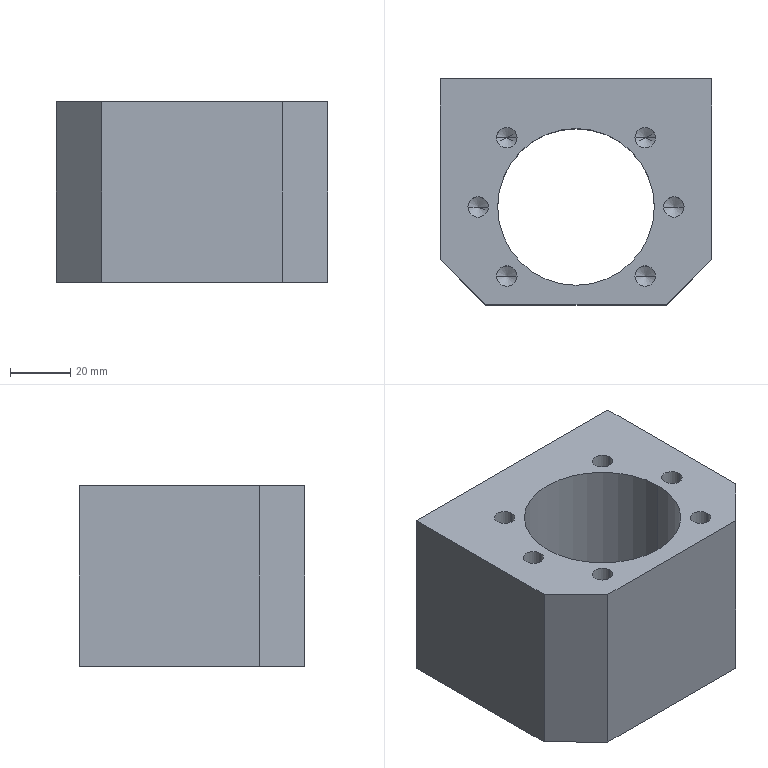Part | SolidWorks | features 3DProfileFeature 2, HoleWzd 2, Chamfer 1, Extrusion 1 | 1 solid | 50 faces | box 90 x 75 x 60 mm | volume 256657 mm3 | cylinder 22 | cone 20 | plane 8 | commonest cylinder face diameters 6.8 x20 52 x2
STEP:
#1=CARTESIAN_POINT('',(32.5,22.75,-23.4));
#2=VERTEX_POINT('',#1);
#3=CARTESIAN_POINT('',(32.5,22.75,-16.6));
#4=VERTEX_POINT('',#3);
#5=CARTESIAN_POINT('',(32.5,22.75,-20.));
#6=DIRECTION('',(0.,1.,0.));
#7=DIRECTION('',(0.,0.,1.));
#8=AXIS2_PLACEMENT_3D('',#5,#6,#7);
#9=CIRCLE('',#8,3.4);
#10=EDGE_CURVE('',#2,#4,#9,.T.);
#11=ORIENTED_EDGE('',*,*,#10,.F.);
#12=CARTESIAN_POINT('',(32.5,42.5,-23.4));
#13=VERTEX_POINT('',#12);
#14=CARTESIAN_POINT('',(32.5,42.5,-23.4));
#15=DIRECTION('',(0.,1.,0.));
#16=VECTOR('',#15,1000.);
#17=LINE('',#14,#16);
#18=EDGE_CURVE('',#2,#13,#17,.T.);
#19=ORIENTED_EDGE('',*,*,#18,.T.);
#20=CARTESIAN_POINT('',(32.5,42.5,-16.6));
#21=VERTEX_POINT('',#20);
#22=CARTESIAN_POINT('',(32.5,42.5,-20.));
#23=DIRECTION('',(0.,1.,0.));
#24=DIRECTION('',(0.,0.,1.));
#25=AXIS2_PLACEMENT_3D('',#22,#23,#24);
#26=CIRCLE('',#25,3.4);
#27=EDGE_CURVE('',#13,#21,#26,.T.);
#28=ORIENTED_EDGE('',*,*,#27,.T.);
#29=CARTESIAN_POINT('',(32.5,42.5,-16.6));
#30=DIRECTION('',(0.,1.,0.));
#31=VECTOR('',#30,1000.);
#32=LINE('',#29,#31);
#33=EDGE_CURVE('',#4,#21,#32,.T.);
#34=ORIENTED_EDGE('',*,*,#33,.F.);
#35=EDGE_LOOP('',(#11,#19,#28,#34));
#36=FACE_OUTER_BOUND('',#35,.T.);
#37=CARTESIAN_POINT('',(32.5,42.5,-20.));
#38=DIRECTION('',(0.,1.,0.));
#39=DIRECTION('',(0.,0.,1.));
#40=AXIS2_PLACEMENT_3D('',#37,#38,#39);
#41=CYLINDRICAL_SURFACE('',#40,3.4);
#42=ADVANCED_FACE('',(#36),#41,.F.);
#43=CARTESIAN_POINT('',(32.5,20.707,-20.));
#44=VERTEX_POINT('',#43);
#45=CARTESIAN_POINT('',(32.5,22.75,-16.6));
#46=DIRECTION('',(0.,0.515,0.8572));
#47=VECTOR('',#46,1000.);
#48=LINE('',#45,#47);
#49=EDGE_CURVE('',#44,#4,#48,.T.);
#50=ORIENTED_EDGE('',*,*,#49,.F.);
#51=CARTESIAN_POINT('',(32.5,22.75,-23.4));
#52=DIRECTION('',(0.,0.515,-0.8572));
#53=VECTOR('',#52,1000.);
#54=LINE('',#51,#53);
#55=EDGE_CURVE('',#44,#2,#54,.T.);
#56=ORIENTED_EDGE('',*,*,#55,.T.);
#57=ORIENTED_EDGE('',*,*,#10,.T.);
#58=EDGE_LOOP('',(#50,#56,#57));
#59=FACE_OUTER_BOUND('',#58,.T.);
#60=CARTESIAN_POINT('',(32.5,22.75,-20.));
#61=DIRECTION('',(0.,1.,0.));
#62=DIRECTION('',(0.,0.,1.));
#63=AXIS2_PLACEMENT_3D('',#60,#61,#62);
#64=CONICAL_SURFACE('',#63,3.4,1.03);
#65=ADVANCED_FACE('',(#59),#64,.F.);
#66=CARTESIAN_POINT('',(32.5,22.75,16.6));
#67=VERTEX_POINT('',#66);
#68=CARTESIAN_POINT('',(32.5,22.75,23.4));
#69=VERTEX_POINT('',#68);
#70=CARTESIAN_POINT('',(32.5,22.75,20.));
#71=DIRECTION('',(0.,1.,0.));
#72=DIRECTION('',(0.,0.,1.));
#73=AXIS2_PLACEMENT_3D('',#70,#71,#72);
#74=CIRCLE('',#73,3.4);
#75=EDGE_CURVE('',#67,#69,#74,.T.);
#76=ORIENTED_EDGE('',*,*,#75,.F.);
#77=CARTESIAN_POINT('',(32.5,42.5,16.6));
#78=VERTEX_POINT('',#77);
#79=CARTESIAN_POINT('',(32.5,42.5,16.6));
#80=DIRECTION('',(0.,1.,0.));
#81=VECTOR('',#80,1000.);
#82=LINE('',#79,#81);
#83=EDGE_CURVE('',#67,#78,#82,.T.);
#84=ORIENTED_EDGE('',*,*,#83,.T.);
#85=CARTESIAN_POINT('',(32.5,42.5,23.4));
#86=VERTEX_POINT('',#85);
#87=CARTESIAN_POINT('',(32.5,42.5,20.));
#88=DIRECTION('',(0.,1.,0.));
#89=DIRECTION('',(0.,0.,1.));
#90=AXIS2_PLACEMENT_3D('',#87,#88,#89);
#91=CIRCLE('',#90,3.4);
#92=EDGE_CURVE('',#78,#86,#91,.T.);
#93=ORIENTED_EDGE('',*,*,#92,.T.);
#94=CARTESIAN_POINT('',(32.5,42.5,23.4));
#95=DIRECTION('',(0.,1.,0.));
#96=VECTOR('',#95,1000.);
#97=LINE('',#94,#96);
#98=EDGE_CURVE('',#69,#86,#97,.T.);
#99=ORIENTED_EDGE('',*,*,#98,.F.);
#100=EDGE_LOOP('',(#76,#84,#93,#99));
#101=FACE_OUTER_BOUND('',#100,.T.);
#102=CARTESIAN_POINT('',(32.5,42.5,20.));
#103=DIRECTION('',(0.,1.,0.));
#104=DIRECTION('',(0.,0.,1.));
#105=AXIS2_PLACEMENT_3D('',#102,#103,#104);
#106=CYLINDRICAL_SURFACE('',#105,3.4);
#107=ADVANCED_FACE('',(#101),#106,.F.);
#108=CARTESIAN_POINT('',(32.5,20.707,20.));
#109=VERTEX_POINT('',#108);
#110=CARTESIAN_POINT('',(32.5,22.75,23.4));
#111=DIRECTION('',(0.,0.515,0.8572));
#112=VECTOR('',#111,1000.);
#113=LINE('',#110,#112);
#114=EDGE_CURVE('',#109,#69,#113,.T.);
#115=ORIENTED_EDGE('',*,*,#114,.F.);
#116=CARTESIAN_POINT('',(32.5,22.75,16.6));
#117=DIRECTION('',(0.,0.515,-0.8572));
#118=VECTOR('',#117,1000.);
#119=LINE('',#116,#118);
#120=EDGE_CURVE('',#109,#67,#119,.T.);
#121=ORIENTED_EDGE('',*,*,#120,.T.);
#122=ORIENTED_EDGE('',*,*,#75,.T.);
#123=EDGE_LOOP('',(#115,#121,#122));
#124=FACE_OUTER_BOUND('',#123,.T.);
#125=CARTESIAN_POINT('',(32.5,22.75,20.));
#126=DIRECTION('',(0.,1.,0.));
#127=DIRECTION('',(0.,0.,1.));
#128=AXIS2_PLACEMENT_3D('',#125,#126,#127);
#129=CONICAL_SURFACE('',#128,3.4,1.03);
#130=ADVANCED_FACE('',(#124),#129,.F.);
#131=CARTESIAN_POINT('',(-32.5,22.75,16.6));
#132=VERTEX_POINT('',#131);
#133=CARTESIAN_POINT('',(-32.5,22.75,23.4));
#134=VERTEX_POINT('',#133);
#135=CARTESIAN_POINT('',(-32.5,22.75,20.));
#136=DIRECTION('',(0.,1.,0.));
#137=DIRECTION('',(0.,0.,1.));
#138=AXIS2_PLACEMENT_3D('',#135,#136,#137);
#139=CIRCLE('',#138,3.4);
#140=EDGE_CURVE('',#132,#134,#139,.T.);
#141=ORIENTED_EDGE('',*,*,#140,.F.);
#142=CARTESIAN_POINT('',(-32.5,42.5,16.6));
#143=VERTEX_POINT('',#142);
#144=CARTESIAN_POINT('',(-32.5,42.5,16.6));
#145=DIRECTION('',(0.,1.,0.));
#146=VECTOR('',#145,1000.);
#147=LINE('',#144,#146);
#148=EDGE_CURVE('',#132,#143,#147,.T.);
#149=ORIENTED_EDGE('',*,*,#148,.T.);
#150=CARTESIAN_POINT('',(-32.5,42.5,23.4));
#151=VERTEX_POINT('',#150);
#152=CARTESIAN_POINT('',(-32.5,42.5,20.));
#153=DIRECTION('',(0.,1.,0.));
#154=DIRECTION('',(0.,0.,1.));
#155=AXIS2_PLACEMENT_3D('',#152,#153,#154);
#156=CIRCLE('',#155,3.4);
#157=EDGE_CURVE('',#143,#151,#156,.T.);
#158=ORIENTED_EDGE('',*,*,#157,.T.);
#159=CARTESIAN_POINT('',(-32.5,42.5,23.4));
#160=DIRECTION('',(0.,1.,0.));
#161=VECTOR('',#160,1000.);
#162=LINE('',#159,#161);
#163=EDGE_CURVE('',#134,#151,#162,.T.);
#164=ORIENTED_EDGE('',*,*,#163,.F.);
#165=EDGE_LOOP('',(#141,#149,#158,#164));
#166=FACE_OUTER_BOUND('',#165,.T.);
#167=CARTESIAN_POINT('',(-32.5,42.5,20.));
#168=DIRECTION('',(0.,1.,0.));
#169=DIRECTION('',(0.,0.,1.));
#170=AXIS2_PLACEMENT_3D('',#167,#168,#169);
#171=CYLINDRICAL_SURFACE('',#170,3.4);
#172=ADVANCED_FACE('',(#166),#171,.F.);
#173=CARTESIAN_POINT('',(-32.5,20.707,20.));
#174=VERTEX_POINT('',#173);
#175=CARTESIAN_POINT('',(-32.5,22.75,23.4));
#176=DIRECTION('',(0.,0.515,0.8572));
#177=VECTOR('',#176,1000.);
#178=LINE('',#175,#177);
#179=EDGE_CURVE('',#174,#134,#178,.T.);
#180=ORIENTED_EDGE('',*,*,#179,.F.);
#181=CARTESIAN_POINT('',(-32.5,22.75,16.6));
#182=DIRECTION('',(0.,0.515,-0.8572));
#183=VECTOR('',#182,1000.);
#184=LINE('',#181,#183);
#185=EDGE_CURVE('',#174,#132,#184,.T.);
#186=ORIENTED_EDGE('',*,*,#185,.T.);
#187=ORIENTED_EDGE('',*,*,#140,.T.);
#188=EDGE_LOOP('',(#180,#186,#187));
#189=FACE_OUTER_BOUND('',#188,.T.);
#190=CARTESIAN_POINT('',(-32.5,22.75,20.));
#191=DIRECTION('',(0.,1.,0.));
#192=DIRECTION('',(0.,0.,1.));
#193=AXIS2_PLACEMENT_3D('',#190,#191,#192);
#194=CONICAL_SURFACE('',#193,3.4,1.03);
#195=ADVANCED_FACE('',(#189),#194,.F.);
#196=CARTESIAN_POINT('',(-32.5,22.75,-23.4));
#197=VERTEX_POINT('',#196);
#198=CARTESIAN_POINT('',(-32.5,22.75,-16.6));
#199=VERTEX_POINT('',#198);
#200=CARTESIAN_POINT('',(-32.5,22.75,-20.));
#201=DIRECTION('',(0.,1.,0.));
#202=DIRECTION('',(0.,0.,1.));
#203=AXIS2_PLACEMENT_3D('',#200,#201,#202);
#204=CIRCLE('',#203,3.4);
#205=EDGE_CURVE('',#197,#199,#204,.T.);
#206=ORIENTED_EDGE('',*,*,#205,.F.);
#207=CARTESIAN_POINT('',(-32.5,42.5,-23.4));
#208=VERTEX_POINT('',#207);
#209=CARTESIAN_POINT('',(-32.5,42.5,-23.4));
#210=DIRECTION('',(0.,1.,0.));
#211=VECTOR('',#210,1000.);
#212=LINE('',#209,#211);
#213=EDGE_CURVE('',#197,#208,#212,.T.);
#214=ORIENTED_EDGE('',*,*,#213,.T.);
#215=CARTESIAN_POINT('',(-32.5,42.5,-16.6));
#216=VERTEX_POINT('',#215);
#217=CARTESIAN_POINT('',(-32.5,42.5,-20.));
#218=DIRECTION('',(0.,1.,0.));
#219=DIRECTION('',(0.,0.,1.));
#220=AXIS2_PLACEMENT_3D('',#217,#218,#219);
#221=CIRCLE('',#220,3.4);
#222=EDGE_CURVE('',#208,#216,#221,.T.);
#223=ORIENTED_EDGE('',*,*,#222,.T.);
#224=CARTESIAN_POINT('',(-32.5,42.5,-16.6));
#225=DIRECTION('',(0.,1.,0.));
#226=VECTOR('',#225,1000.);
#227=LINE('',#224,#226);
#228=EDGE_CURVE('',#199,#216,#227,.T.);
#229=ORIENTED_EDGE('',*,*,#228,.F.);
#230=EDGE_LOOP('',(#206,#214,#223,#229));
#231=FACE_OUTER_BOUND('',#230,.T.);
#232=CARTESIAN_POINT('',(-32.5,42.5,-20.));
#233=DIRECTION('',(0.,1.,0.));
#234=DIRECTION('',(0.,0.,1.));
#235=AXIS2_PLACEMENT_3D('',#232,#233,#234);
#236=CYLINDRICAL_SURFACE('',#235,3.4);
#237=ADVANCED_FACE('',(#231),#236,.F.);
#238=CARTESIAN_POINT('',(-32.5,20.707,-20.));
#239=VERTEX_POINT('',#238);
#240=CARTESIAN_POINT('',(-32.5,22.75,-16.6));
#241=DIRECTION('',(0.,0.515,0.8572));
#242=VECTOR('',#241,1000.);
#243=LINE('',#240,#242);
#244=EDGE_CURVE('',#239,#199,#243,.T.);
#245=ORIENTED_EDGE('',*,*,#244,.F.);
#246=CARTESIAN_POINT('',(-32.5,22.75,-23.4));
#247=DIRECTION('',(0.,0.515,-0.8572));
#248=VECTOR('',#247,1000.);
#249=LINE('',#246,#248);
#250=EDGE_CURVE('',#239,#197,#249,.T.);
#251=ORIENTED_EDGE('',*,*,#250,.T.);
#252=ORIENTED_EDGE('',*,*,#205,.T.);
#253=EDGE_LOOP('',(#245,#251,#252));
#254=FACE_OUTER_BOUND('',#253,.T.);
#255=CARTESIAN_POINT('',(-32.5,22.75,-20.));
#256=DIRECTION('',(0.,1.,0.));
#257=DIRECTION('',(0.,0.,1.));
#258=AXIS2_PLACEMENT_3D('',#255,#256,#257);
#259=CONICAL_SURFACE('',#258,3.4,1.03);
#260=ADVANCED_FACE('',(#254),#259,.F.);
#261=CARTESIAN_POINT('',(-35.9,0.,10.25));
#262=VERTEX_POINT('',#261);
#263=CARTESIAN_POINT('',(-29.1,0.,10.25));
#264=VERTEX_POINT('',#263);
#265=CARTESIAN_POINT('',(-32.5,0.,10.25));
#266=DIRECTION('',(0.,0.,1.));
#267=DIRECTION('',(1.,0.,0.));
#268=AXIS2_PLACEMENT_3D('',#265,#266,#267);
#269=CIRCLE('',#268,3.4);
#270=EDGE_CURVE('',#262,#264,#269,.T.);
#271=ORIENTED_EDGE('',*,*,#270,.F.);
#272=CARTESIAN_POINT('',(-35.9,0.,30.));
#273=VERTEX_POINT('',#272);
#274=CARTESIAN_POINT('',(-35.9,0.,30.));
#275=DIRECTION('',(0.,0.,1.));
#276=VECTOR('',#275,1000.);
#277=LINE('',#274,#276);
#278=EDGE_CURVE('',#262,#273,#277,.T.);
#279=ORIENTED_EDGE('',*,*,#278,.T.);
#280=CARTESIAN_POINT('',(-29.1,0.,30.));
#281=VERTEX_POINT('',#280);
#282=CARTESIAN_POINT('',(-32.5,0.,30.));
#283=DIRECTION('',(0.,0.,1.));
#284=DIRECTION('',(1.,0.,0.));
#285=AXIS2_PLACEMENT_3D('',#282,#283,#284);
#286=CIRCLE('',#285,3.4);
#287=EDGE_CURVE('',#273,#281,#286,.T.);
#288=ORIENTED_EDGE('',*,*,#287,.T.);
#289=CARTESIAN_POINT('',(-29.1,0.,30.));
#290=DIRECTION('',(0.,0.,1.));
#291=VECTOR('',#290,1000.);
#292=LINE('',#289,#291);
#293=EDGE_CURVE('',#264,#281,#292,.T.);
#294=ORIENTED_EDGE('',*,*,#293,.F.);
#295=EDGE_LOOP('',(#271,#279,#288,#294));
#296=FACE_OUTER_BOUND('',#295,.T.);
#297=CARTESIAN_POINT('',(-32.5,0.,30.));
#298=DIRECTION('',(0.,0.,1.));
#299=DIRECTION('',(1.,0.,0.));
#300=AXIS2_PLACEMENT_3D('',#297,#298,#299);
#301=CYLINDRICAL_SURFACE('',#300,3.4);
#302=ADVANCED_FACE('',(#296),#301,.F.);
#303=CARTESIAN_POINT('',(-32.5,0.,8.207));
#304=VERTEX_POINT('',#303);
#305=CARTESIAN_POINT('',(-29.1,0.,10.25));
#306=DIRECTION('',(0.8572,0.,0.515));
#307=VECTOR('',#306,1000.);
#308=LINE('',#305,#307);
#309=EDGE_CURVE('',#304,#264,#308,.T.);
#310=ORIENTED_EDGE('',*,*,#309,.F.);
#311=CARTESIAN_POINT('',(-35.9,0.,10.25));
#312=DIRECTION('',(-0.8572,0.,0.515));
#313=VECTOR('',#312,1000.);
#314=LINE('',#311,#313);
#315=EDGE_CURVE('',#304,#262,#314,.T.);
#316=ORIENTED_EDGE('',*,*,#315,.T.);
#317=ORIENTED_EDGE('',*,*,#270,.T.);
#318=EDGE_LOOP('',(#310,#316,#317));
#319=FACE_OUTER_BOUND('',#318,.T.);
#320=CARTESIAN_POINT('',(-32.5,0.,10.25));
#321=DIRECTION('',(0.,0.,1.));
#322=DIRECTION('',(1.,0.,0.));
#323=AXIS2_PLACEMENT_3D('',#320,#321,#322);
#324=CONICAL_SURFACE('',#323,3.4,1.03);
#325=ADVANCED_FACE('',(#319),#324,.F.);
#326=CARTESIAN_POINT('',(-26.381,22.981,10.25));
#327=VERTEX_POINT('',#326);
#328=CARTESIAN_POINT('',(-19.581,22.981,10.25));
#329=VERTEX_POINT('',#328);
#330=CARTESIAN_POINT('',(-22.981,22.981,10.25));
#331=DIRECTION('',(0.,0.,1.));
#332=DIRECTION('',(1.,0.,0.));
#333=AXIS2_PLACEMENT_3D('',#330,#331,#332);
#334=CIRCLE('',#333,3.4);
#335=EDGE_CURVE('',#327,#329,#334,.T.);
#336=ORIENTED_EDGE('',*,*,#335,.F.);
#337=CARTESIAN_POINT('',(-26.381,22.981,30.));
#338=VERTEX_POINT('',#337);
#339=CARTESIAN_POINT('',(-26.381,22.981,30.));
#340=DIRECTION('',(0.,0.,1.));
#341=VECTOR('',#340,1000.);
#342=LINE('',#339,#341);
#343=EDGE_CURVE('',#327,#338,#342,.T.);
#344=ORIENTED_EDGE('',*,*,#343,.T.);
#345=CARTESIAN_POINT('',(-19.581,22.981,30.));
#346=VERTEX_POINT('',#345);
#347=CARTESIAN_POINT('',(-22.981,22.981,30.));
#348=DIRECTION('',(0.,0.,1.));
#349=DIRECTION('',(1.,0.,0.));
#350=AXIS2_PLACEMENT_3D('',#347,#348,#349);
#351=CIRCLE('',#350,3.4);
#352=EDGE_CURVE('',#338,#346,#351,.T.);
#353=ORIENTED_EDGE('',*,*,#352,.T.);
#354=CARTESIAN_POINT('',(-19.581,22.981,30.));
#355=DIRECTION('',(0.,0.,1.));
#356=VECTOR('',#355,1000.);
#357=LINE('',#354,#356);
#358=EDGE_CURVE('',#329,#346,#357,.T.);
#359=ORIENTED_EDGE('',*,*,#358,.F.);
#360=EDGE_LOOP('',(#336,#344,#353,#359));
#361=FACE_OUTER_BOUND('',#360,.T.);
#362=CARTESIAN_POINT('',(-22.981,22.981,30.));
#363=DIRECTION('',(0.,0.,1.));
#364=DIRECTION('',(1.,0.,0.));
#365=AXIS2_PLACEMENT_3D('',#362,#363,#364);
#366=CYLINDRICAL_SURFACE('',#365,3.4);
#367=ADVANCED_FACE('',(#361),#366,.F.);
#368=CARTESIAN_POINT('',(-22.981,22.981,8.207));
#369=VERTEX_POINT('',#368);
#370=CARTESIAN_POINT('',(-19.581,22.981,10.25));
#371=DIRECTION('',(0.8572,0.,0.515));
#372=VECTOR('',#371,1000.);
#373=LINE('',#370,#372);
#374=EDGE_CURVE('',#369,#329,#373,.T.);
#375=ORIENTED_EDGE('',*,*,#374,.F.);
#376=CARTESIAN_POINT('',(-26.381,22.981,10.25));
#377=DIRECTION('',(-0.8572,0.,0.515));
#378=VECTOR('',#377,1000.);
#379=LINE('',#376,#378);
#380=EDGE_CURVE('',#369,#327,#379,.T.);
#381=ORIENTED_EDGE('',*,*,#380,.T.);
#382=ORIENTED_EDGE('',*,*,#335,.T.);
#383=EDGE_LOOP('',(#375,#381,#382));
#384=FACE_OUTER_BOUND('',#383,.T.);
#385=CARTESIAN_POINT('',(-22.981,22.981,10.25));
#386=DIRECTION('',(0.,0.,1.));
#387=DIRECTION('',(1.,0.,0.));
#388=AXIS2_PLACEMENT_3D('',#385,#386,#387);
#389=CONICAL_SURFACE('',#388,3.4,1.03);
#390=ADVANCED_FACE('',(#384),#389,.F.);
#391=CARTESIAN_POINT('',(-26.381,-22.981,10.25));
#392=VERTEX_POINT('',#391);
#393=CARTESIAN_POINT('',(-19.581,-22.981,10.25));
#394=VERTEX_POINT('',#393);
#395=CARTESIAN_POINT('',(-22.981,-22.981,10.25));
#396=DIRECTION('',(0.,0.,1.));
#397=DIRECTION('',(1.,0.,0.));
#398=AXIS2_PLACEMENT_3D('',#395,#396,#397);
#399=CIRCLE('',#398,3.4);
#400=EDGE_CURVE('',#392,#394,#399,.T.);
#401=ORIENTED_EDGE('',*,*,#400,.F.);
#402=CARTESIAN_POINT('',(-26.381,-22.981,30.));
#403=VERTEX_POINT('',#402);
#404=CARTESIAN_POINT('',(-26.381,-22.981,30.));
#405=DIRECTION('',(0.,0.,1.));
#406=VECTOR('',#405,1000.);
#407=LINE('',#404,#406);
#408=EDGE_CURVE('',#392,#403,#407,.T.);
#409=ORIENTED_EDGE('',*,*,#408,.T.);
#410=CARTESIAN_POINT('',(-19.581,-22.981,30.));
#411=VERTEX_POINT('',#410);
#412=CARTESIAN_POINT('',(-22.981,-22.981,30.));
#413=DIRECTION('',(0.,0.,1.));
#414=DIRECTION('',(1.,0.,0.));
#415=AXIS2_PLACEMENT_3D('',#412,#413,#414);
#416=CIRCLE('',#415,3.4);
#417=EDGE_CURVE('',#403,#411,#416,.T.);
#418=ORIENTED_EDGE('',*,*,#417,.T.);
#419=CARTESIAN_POINT('',(-19.581,-22.981,30.));
#420=DIRECTION('',(0.,0.,1.));
#421=VECTOR('',#420,1000.);
#422=LINE('',#419,#421);
#423=EDGE_CURVE('',#394,#411,#422,.T.);
#424=ORIENTED_EDGE('',*,*,#423,.F.);
#425=EDGE_LOOP('',(#401,#409,#418,#424));
#426=FACE_OUTER_BOUND('',#425,.T.);
#427=CARTESIAN_POINT('',(-22.981,-22.981,30.));
#428=DIRECTION('',(0.,0.,1.));
#429=DIRECTION('',(1.,0.,0.));
#430=AXIS2_PLACEMENT_3D('',#427,#428,#429);
#431=CYLINDRICAL_SURFACE('',#430,3.4);
#432=ADVANCED_FACE('',(#426),#431,.F.);
#433=CARTESIAN_POINT('',(-22.981,-22.981,8.207));
#434=VERTEX_POINT('',#433);
#435=CARTESIAN_POINT('',(-19.581,-22.981,10.25));
#436=DIRECTION('',(0.8572,0.,0.515));
#437=VECTOR('',#436,1000.);
#438=LINE('',#435,#437);
#439=EDGE_CURVE('',#434,#394,#438,.T.);
#440=ORIENTED_EDGE('',*,*,#439,.F.);
#441=CARTESIAN_POINT('',(-26.381,-22.981,10.25));
#442=DIRECTION('',(-0.8572,0.,0.515));
#443=VECTOR('',#442,1000.);
#444=LINE('',#441,#443);
#445=EDGE_CURVE('',#434,#392,#444,.T.);
#446=ORIENTED_EDGE('',*,*,#445,.T.);
#447=ORIENTED_EDGE('',*,*,#400,.T.);
#448=EDGE_LOOP('',(#440,#446,#447));
#449=FACE_OUTER_BOUND('',#448,.T.);
#450=CARTESIAN_POINT('',(-22.981,-22.981,10.25));
#451=DIRECTION('',(0.,0.,1.));
#452=DIRECTION('',(1.,0.,0.));
#453=AXIS2_PLACEMENT_3D('',#450,#451,#452);
#454=CONICAL_SURFACE('',#453,3.4,1.03);
#455=ADVANCED_FACE('',(#449),#454,.F.);
#456=CARTESIAN_POINT('',(19.581,-22.981,10.25));
#457=VERTEX_POINT('',#456);
#458=CARTESIAN_POINT('',(26.381,-22.981,10.25));
#459=VERTEX_POINT('',#458);
#460=CARTESIAN_POINT('',(22.981,-22.981,10.25));
#461=DIRECTION('',(0.,0.,1.));
#462=DIRECTION('',(1.,0.,0.));
#463=AXIS2_PLACEMENT_3D('',#460,#461,#462);
#464=CIRCLE('',#463,3.4);
#465=EDGE_CURVE('',#457,#459,#464,.T.);
#466=ORIENTED_EDGE('',*,*,#465,.F.);
#467=CARTESIAN_POINT('',(19.581,-22.981,30.));
#468=VERTEX_POINT('',#467);
#469=CARTESIAN_POINT('',(19.581,-22.981,30.));
#470=DIRECTION('',(0.,0.,1.));
#471=VECTOR('',#470,1000.);
#472=LINE('',#469,#471);
#473=EDGE_CURVE('',#457,#468,#472,.T.);
#474=ORIENTED_EDGE('',*,*,#473,.T.);
#475=CARTESIAN_POINT('',(26.381,-22.981,30.));
#476=VERTEX_POINT('',#475);
#477=CARTESIAN_POINT('',(22.981,-22.981,30.));
#478=DIRECTION('',(0.,0.,1.));
#479=DIRECTION('',(1.,0.,0.));
#480=AXIS2_PLACEMENT_3D('',#477,#478,#479);
#481=CIRCLE('',#480,3.4);
#482=EDGE_CURVE('',#468,#476,#481,.T.);
#483=ORIENTED_EDGE('',*,*,#482,.T.);
#484=CARTESIAN_POINT('',(26.381,-22.981,30.));
#485=DIRECTION('',(0.,0.,1.));
#486=VECTOR('',#485,1000.);
#487=LINE('',#484,#486);
#488=EDGE_CURVE('',#459,#476,#487,.T.);
#489=ORIENTED_EDGE('',*,*,#488,.F.);
#490=EDGE_LOOP('',(#466,#474,#483,#489));
#491=FACE_OUTER_BOUND('',#490,.T.);
#492=CARTESIAN_POINT('',(22.981,-22.981,30.));
#493=DIRECTION('',(0.,0.,1.));
#494=DIRECTION('',(1.,0.,0.));
#495=AXIS2_PLACEMENT_3D('',#492,#493,#494);
#496=CYLINDRICAL_SURFACE('',#495,3.4);
#497=ADVANCED_FACE('',(#491),#496,.F.);
#498=CARTESIAN_POINT('',(22.981,-22.981,8.207));
#499=VERTEX_POINT('',#498);
#500=CARTESIAN_POINT('',(26.381,-22.981,10.25));
#501=DIRECTION('',(0.8572,0.,0.515));
#502=VECTOR('',#501,1000.);
#503=LINE('',#500,#502);
#504=EDGE_CURVE('',#499,#459,#503,.T.);
#505=ORIENTED_EDGE('',*,*,#504,.F.);
#506=CARTESIAN_POINT('',(19.581,-22.981,10.25));
#507=DIRECTION('',(-0.8572,0.,0.515));
#508=VECTOR('',#507,1000.);
#509=LINE('',#506,#508);
#510=EDGE_CURVE('',#499,#457,#509,.T.);
#511=ORIENTED_EDGE('',*,*,#510,.T.);
#512=ORIENTED_EDGE('',*,*,#465,.T.);
#513=EDGE_LOOP('',(#505,#511,#512));
#514=FACE_OUTER_BOUND('',#513,.T.);
#515=CARTESIAN_POINT('',(22.981,-22.981,10.25));
#516=DIRECTION('',(0.,0.,1.));
#517=DIRECTION('',(1.,0.,0.));
#518=AXIS2_PLACEMENT_3D('',#515,#516,#517);
#519=CONICAL_SURFACE('',#518,3.4,1.03);
#520=ADVANCED_FACE('',(#514),#519,.F.);
#521=CARTESIAN_POINT('',(29.1,0.,10.25));
#522=VERTEX_POINT('',#521);
#523=CARTESIAN_POINT('',(35.9,0.,10.25));
#524=VERTEX_POINT('',#523);
#525=CARTESIAN_POINT('',(32.5,0.,10.25));
#526=DIRECTION('',(0.,0.,1.));
#527=DIRECTION('',(1.,0.,0.));
#528=AXIS2_PLACEMENT_3D('',#525,#526,#527);
#529=CIRCLE('',#528,3.4);
#530=EDGE_CURVE('',#522,#524,#529,.T.);
#531=ORIENTED_EDGE('',*,*,#530,.F.);
#532=CARTESIAN_POINT('',(29.1,0.,30.));
#533=VERTEX_POINT('',#532);
#534=CARTESIAN_POINT('',(29.1,0.,30.));
#535=DIRECTION('',(0.,0.,1.));
#536=VECTOR('',#535,1000.);
#537=LINE('',#534,#536);
#538=EDGE_CURVE('',#522,#533,#537,.T.);
#539=ORIENTED_EDGE('',*,*,#538,.T.);
#540=CARTESIAN_POINT('',(35.9,0.,30.));
#541=VERTEX_POINT('',#540);
#542=CARTESIAN_POINT('',(32.5,0.,30.));
#543=DIRECTION('',(0.,0.,1.));
#544=DIRECTION('',(1.,0.,0.));
#545=AXIS2_PLACEMENT_3D('',#542,#543,#544);
#546=CIRCLE('',#545,3.4);
#547=EDGE_CURVE('',#533,#541,#546,.T.);
#548=ORIENTED_EDGE('',*,*,#547,.T.);
#549=CARTESIAN_POINT('',(35.9,0.,30.));
#550=DIRECTION('',(0.,0.,1.));
#551=VECTOR('',#550,1000.);
#552=LINE('',#549,#551);
#553=EDGE_CURVE('',#524,#541,#552,.T.);
#554=ORIENTED_EDGE('',*,*,#553,.F.);
#555=EDGE_LOOP('',(#531,#539,#548,#554));
#556=FACE_OUTER_BOUND('',#555,.T.);
#557=CARTESIAN_POINT('',(32.5,0.,30.));
#558=DIRECTION('',(0.,0.,1.));
#559=DIRECTION('',(1.,0.,0.));
#560=AXIS2_PLACEMENT_3D('',#557,#558,#559);
#561=CYLINDRICAL_SURFACE('',#560,3.4);
#562=ADVANCED_FACE('',(#556),#561,.F.);
#563=CARTESIAN_POINT('',(32.5,0.,8.207));
#564=VERTEX_POINT('',#563);
#565=CARTESIAN_POINT('',(35.9,0.,10.25));
#566=DIRECTION('',(0.8572,0.,0.515));
#567=VECTOR('',#566,1000.);
#568=LINE('',#565,#567);
#569=EDGE_CURVE('',#564,#524,#568,.T.);
#570=ORIENTED_EDGE('',*,*,#569,.F.);
#571=CARTESIAN_POINT('',(29.1,0.,10.25));
#572=DIRECTION('',(-0.8572,0.,0.515));
#573=VECTOR('',#572,1000.);
#574=LINE('',#571,#573);
#575=EDGE_CURVE('',#564,#522,#574,.T.);
#576=ORIENTED_EDGE('',*,*,#575,.T.);
#577=ORIENTED_EDGE('',*,*,#530,.T.);
#578=EDGE_LOOP('',(#570,#576,#577));
#579=FACE_OUTER_BOUND('',#578,.T.);
#580=CARTESIAN_POINT('',(32.5,0.,10.25));
#581=DIRECTION('',(0.,0.,1.));
#582=DIRECTION('',(1.,0.,0.));
#583=AXIS2_PLACEMENT_3D('',#580,#581,#582);
#584=CONICAL_SURFACE('',#583,3.4,1.03);
#585=ADVANCED_FACE('',(#579),#584,.F.);
#586=CARTESIAN_POINT('',(19.581,22.981,10.25));
#587=VERTEX_POINT('',#586);
#588=CARTESIAN_POINT('',(26.381,22.981,10.25));
#589=VERTEX_POINT('',#588);
#590=CARTESIAN_POINT('',(22.981,22.981,10.25));
#591=DIRECTION('',(0.,0.,1.));
#592=DIRECTION('',(1.,0.,0.));
#593=AXIS2_PLACEMENT_3D('',#590,#591,#592);
#594=CIRCLE('',#593,3.4);
#595=EDGE_CURVE('',#587,#589,#594,.T.);
#596=ORIENTED_EDGE('',*,*,#595,.F.);
#597=CARTESIAN_POINT('',(19.581,22.981,30.));
#598=VERTEX_POINT('',#597);
#599=CARTESIAN_POINT('',(19.581,22.981,30.));
#600=DIRECTION('',(0.,0.,1.));
#601=VECTOR('',#600,1000.);
#602=LINE('',#599,#601);
#603=EDGE_CURVE('',#587,#598,#602,.T.);
#604=ORIENTED_EDGE('',*,*,#603,.T.);
#605=CARTESIAN_POINT('',(26.381,22.981,30.));
#606=VERTEX_POINT('',#605);
#607=CARTESIAN_POINT('',(22.981,22.981,30.));
#608=DIRECTION('',(0.,0.,1.));
#609=DIRECTION('',(1.,0.,0.));
#610=AXIS2_PLACEMENT_3D('',#607,#608,#609);
#611=CIRCLE('',#610,3.4);
#612=EDGE_CURVE('',#598,#606,#611,.T.);
#613=ORIENTED_EDGE('',*,*,#612,.T.);
#614=CARTESIAN_POINT('',(26.381,22.981,30.));
#615=DIRECTION('',(0.,0.,1.));
#616=VECTOR('',#615,1000.);
#617=LINE('',#614,#616);
#618=EDGE_CURVE('',#589,#606,#617,.T.);
#619=ORIENTED_EDGE('',*,*,#618,.F.);
#620=EDGE_LOOP('',(#596,#604,#613,#619));
#621=FACE_OUTER_BOUND('',#620,.T.);
#622=CARTESIAN_POINT('',(22.981,22.981,30.));
#623=DIRECTION('',(0.,0.,1.));
#624=DIRECTION('',(1.,0.,0.));
#625=AXIS2_PLACEMENT_3D('',#622,#623,#624);
#626=CYLINDRICAL_SURFACE('',#625,3.4);
#627=ADVANCED_FACE('',(#621),#626,.F.);
#628=CARTESIAN_POINT('',(22.981,22.981,8.207));
#629=VERTEX_POINT('',#628);
#630=CARTESIAN_POINT('',(26.381,22.981,10.25));
#631=DIRECTION('',(0.8572,0.,0.515));
#632=VECTOR('',#631,1000.);
#633=LINE('',#630,#632);
#634=EDGE_CURVE('',#629,#589,#633,.T.);
#635=ORIENTED_EDGE('',*,*,#634,.F.);
#636=CARTESIAN_POINT('',(19.581,22.981,10.25));
#637=DIRECTION('',(-0.8572,0.,0.515));
#638=VECTOR('',#637,1000.);
#639=LINE('',#636,#638);
#640=EDGE_CURVE('',#629,#587,#639,.T.);
#641=ORIENTED_EDGE('',*,*,#640,.T.);
#642=ORIENTED_EDGE('',*,*,#595,.T.);
#643=EDGE_LOOP('',(#635,#641,#642));
#644=FACE_OUTER_BOUND('',#643,.T.);
#645=CARTESIAN_POINT('',(22.981,22.981,10.25));
#646=DIRECTION('',(0.,0.,1.));
#647=DIRECTION('',(1.,0.,0.));
#648=AXIS2_PLACEMENT_3D('',#645,#646,#647);
#649=CONICAL_SURFACE('',#648,3.4,1.03);
#650=ADVANCED_FACE('',(#644),#649,.F.);
#651=CARTESIAN_POINT('',(-26.,0.,30.));
#652=VERTEX_POINT('',#651);
#653=CARTESIAN_POINT('',(26.,0.,30.));
#654=VERTEX_POINT('',#653);
#655=CARTESIAN_POINT('',(0.,0.,30.));
#656=DIRECTION('',(0.,0.,1.));
#657=DIRECTION('',(1.,0.,0.));
#658=AXIS2_PLACEMENT_3D('',#655,#656,#657);
#659=CIRCLE('',#658,26.);
#660=EDGE_CURVE('',#652,#654,#659,.T.);
#661=ORIENTED_EDGE('',*,*,#660,.T.);
#662=CARTESIAN_POINT('',(26.,0.,-30.));
#663=VERTEX_POINT('',#662);
#664=CARTESIAN_POINT('',(26.,0.,30.));
#665=DIRECTION('',(0.,0.,-1.));
#666=VECTOR('',#665,1000.);
#667=LINE('',#664,#666);
#668=EDGE_CURVE('',#654,#663,#667,.T.);
#669=ORIENTED_EDGE('',*,*,#668,.T.);
#670=CARTESIAN_POINT('',(-26.,0.,-30.));
#671=VERTEX_POINT('',#670);
#672=CARTESIAN_POINT('',(0.,0.,-30.));
#673=DIRECTION('',(0.,0.,1.));
#674=DIRECTION('',(1.,0.,0.));
#675=AXIS2_PLACEMENT_3D('',#672,#673,#674);
#676=CIRCLE('',#675,26.);
#677=EDGE_CURVE('',#671,#663,#676,.T.);
#678=ORIENTED_EDGE('',*,*,#677,.F.);
#679=CARTESIAN_POINT('',(-26.,0.,30.));
#680=DIRECTION('',(0.,0.,-1.));
#681=VECTOR('',#680,1000.);
#682=LINE('',#679,#681);
#683=EDGE_CURVE('',#652,#671,#682,.T.);
#684=ORIENTED_EDGE('',*,*,#683,.F.);
#685=EDGE_LOOP('',(#661,#669,#678,#684));
#686=FACE_OUTER_BOUND('',#685,.T.);
#687=CARTESIAN_POINT('',(0.,0.,30.));
#688=DIRECTION('',(0.,0.,-1.));
#689=DIRECTION('',(-1.,0.,0.));
#690=AXIS2_PLACEMENT_3D('',#687,#688,#689);
#691=CYLINDRICAL_SURFACE('',#690,26.);
#692=ADVANCED_FACE('',(#686),#691,.F.);
#693=CARTESIAN_POINT('',(-32.5,0.,30.));
#694=DIRECTION('',(0.,0.,1.));
#695=DIRECTION('',(1.,0.,0.));
#696=AXIS2_PLACEMENT_3D('',#693,#694,#695);
#697=CIRCLE('',#696,3.4);
#698=EDGE_CURVE('',#281,#273,#697,.T.);
#699=ORIENTED_EDGE('',*,*,#698,.F.);
#700=ORIENTED_EDGE('',*,*,#287,.F.);
#701=EDGE_LOOP('',(#699,#700));
#702=FACE_BOUND('',#701,.T.);
#703=CARTESIAN_POINT('',(-22.981,22.981,30.));
#704=DIRECTION('',(0.,0.,1.));
#705=DIRECTION('',(1.,0.,0.));
#706=AXIS2_PLACEMENT_3D('',#703,#704,#705);
#707=CIRCLE('',#706,3.4);
#708=EDGE_CURVE('',#346,#338,#707,.T.);
#709=ORIENTED_EDGE('',*,*,#708,.F.);
#710=ORIENTED_EDGE('',*,*,#352,.F.);
#711=EDGE_LOOP('',(#709,#710));
#712=FACE_BOUND('',#711,.T.);
#713=CARTESIAN_POINT('',(-22.981,-22.981,30.));
#714=DIRECTION('',(0.,0.,1.));
#715=DIRECTION('',(1.,0.,0.));
#716=AXIS2_PLACEMENT_3D('',#713,#714,#715);
#717=CIRCLE('',#716,3.4);
#718=EDGE_CURVE('',#411,#403,#717,.T.);
#719=ORIENTED_EDGE('',*,*,#718,.F.);
#720=ORIENTED_EDGE('',*,*,#417,.F.);
#721=EDGE_LOOP('',(#719,#720));
#722=FACE_BOUND('',#721,.T.);
#723=CARTESIAN_POINT('',(22.981,-22.981,30.));
#724=DIRECTION('',(0.,0.,1.));
#725=DIRECTION('',(1.,0.,0.));
#726=AXIS2_PLACEMENT_3D('',#723,#724,#725);
#727=CIRCLE('',#726,3.4);
#728=EDGE_CURVE('',#476,#468,#727,.T.);
#729=ORIENTED_EDGE('',*,*,#728,.F.);
#730=ORIENTED_EDGE('',*,*,#482,.F.);
#731=EDGE_LOOP('',(#729,#730));
#732=FACE_BOUND('',#731,.T.);
#733=CARTESIAN_POINT('',(32.5,0.,30.));
#734=DIRECTION('',(0.,0.,1.));
#735=DIRECTION('',(1.,0.,0.));
#736=AXIS2_PLACEMENT_3D('',#733,#734,#735);
#737=CIRCLE('',#736,3.4);
#738=EDGE_CURVE('',#541,#533,#737,.T.);
#739=ORIENTED_EDGE('',*,*,#738,.F.);
#740=ORIENTED_EDGE('',*,*,#547,.F.);
#741=EDGE_LOOP('',(#739,#740));
#742=FACE_BOUND('',#741,.T.);
#743=CARTESIAN_POINT('',(22.981,22.981,30.));
#744=DIRECTION('',(0.,0.,1.));
#745=DIRECTION('',(1.,0.,0.));
#746=AXIS2_PLACEMENT_3D('',#743,#744,#745);
#747=CIRCLE('',#746,3.4);
#748=EDGE_CURVE('',#606,#598,#747,.T.);
#749=ORIENTED_EDGE('',*,*,#748,.F.);
#750=ORIENTED_EDGE('',*,*,#612,.F.);
#751=EDGE_LOOP('',(#749,#750));
#752=FACE_BOUND('',#751,.T.);
#753=CARTESIAN_POINT('',(-30.,-32.5,30.));
#754=VERTEX_POINT('',#753);
#755=CARTESIAN_POINT('',(30.,-32.5,30.));
#756=VERTEX_POINT('',#755);
#757=CARTESIAN_POINT('',(45.,-32.5,30.));
#758=DIRECTION('',(1.,0.,0.));
#759=VECTOR('',#758,1000.);
#760=LINE('',#757,#759);
#761=EDGE_CURVE('',#754,#756,#760,.T.);
#762=ORIENTED_EDGE('',*,*,#761,.T.);
#763=CARTESIAN_POINT('',(45.,-17.5,30.));
#764=VERTEX_POINT('',#763);
#765=CARTESIAN_POINT('',(31.25,-31.25,30.));
#766=DIRECTION('',(0.7071,0.7071,0.));
#767=VECTOR('',#766,1000.);
#768=LINE('',#765,#767);
#769=EDGE_CURVE('',#756,#764,#768,.T.);
#770=ORIENTED_EDGE('',*,*,#769,.T.);
#771=CARTESIAN_POINT('',(45.,42.5,30.));
#772=VERTEX_POINT('',#771);
#773=CARTESIAN_POINT('',(45.,-32.5,30.));
#774=DIRECTION('',(0.,1.,0.));
#775=VECTOR('',#774,1000.);
#776=LINE('',#773,#775);
#777=EDGE_CURVE('',#764,#772,#776,.T.);
#778=ORIENTED_EDGE('',*,*,#777,.T.);
#779=CARTESIAN_POINT('',(-45.,42.5,30.));
#780=VERTEX_POINT('',#779);
#781=CARTESIAN_POINT('',(45.,42.5,30.));
#782=DIRECTION('',(-1.,0.,0.));
#783=VECTOR('',#782,1000.);
#784=LINE('',#781,#783);
#785=EDGE_CURVE('',#772,#780,#784,.T.);
#786=ORIENTED_EDGE('',*,*,#785,.T.);
#787=CARTESIAN_POINT('',(-45.,-17.5,30.));
#788=VERTEX_POINT('',#787);
#789=CARTESIAN_POINT('',(-45.,-32.5,30.));
#790=DIRECTION('',(0.,-1.,0.));
#791=VECTOR('',#790,1000.);
#792=LINE('',#789,#791);
#793=EDGE_CURVE('',#780,#788,#792,.T.);
#794=ORIENTED_EDGE('',*,*,#793,.T.);
#795=CARTESIAN_POINT('',(-31.25,-31.25,30.));
#796=DIRECTION('',(0.7071,-0.7071,0.));
#797=VECTOR('',#796,1000.);
#798=LINE('',#795,#797);
#799=EDGE_CURVE('',#788,#754,#798,.T.);
#800=ORIENTED_EDGE('',*,*,#799,.T.);
#801=EDGE_LOOP('',(#762,#770,#778,#786,#794,#800));
#802=FACE_OUTER_BOUND('',#801,.T.);
#803=ORIENTED_EDGE('',*,*,#660,.F.);
#804=CARTESIAN_POINT('',(0.,0.,30.));
#805=DIRECTION('',(0.,0.,1.));
#806=DIRECTION('',(1.,0.,0.));
#807=AXIS2_PLACEMENT_3D('',#804,#805,#806);
#808=CIRCLE('',#807,26.);
#809=EDGE_CURVE('',#654,#652,#808,.T.);
#810=ORIENTED_EDGE('',*,*,#809,.F.);
#811=EDGE_LOOP('',(#803,#810));
#812=FACE_BOUND('',#811,.T.);
#813=CARTESIAN_POINT('',(0.,0.,30.));
#814=DIRECTION('',(0.,0.,1.));
#815=DIRECTION('',(1.,0.,0.));
#816=AXIS2_PLACEMENT_3D('',#813,#814,#815);
#817=PLANE('',#816);
#818=ADVANCED_FACE('',(#702,#712,#722,#732,#742,#752,#802,#812),#817,.T.);
#819=CARTESIAN_POINT('',(45.,-17.5,-30.));
#820=VERTEX_POINT('',#819);
#821=CARTESIAN_POINT('',(45.,42.5,-30.));
#822=VERTEX_POINT('',#821);
#823=CARTESIAN_POINT('',(45.,-32.5,-30.));
#824=DIRECTION('',(0.,1.,0.));
#825=VECTOR('',#824,1000.);
#826=LINE('',#823,#825);
#827=EDGE_CURVE('',#820,#822,#826,.T.);
#828=ORIENTED_EDGE('',*,*,#827,.F.);
#829=CARTESIAN_POINT('',(30.,-32.5,-30.));
#830=VERTEX_POINT('',#829);
#831=CARTESIAN_POINT('',(45.,-17.5,-30.));
#832=DIRECTION('',(-0.7071,-0.7071,0.));
#833=VECTOR('',#832,1000.);
#834=LINE('',#831,#833);
#835=EDGE_CURVE('',#820,#830,#834,.T.);
#836=ORIENTED_EDGE('',*,*,#835,.T.);
#837=CARTESIAN_POINT('',(-30.,-32.5,-30.));
#838=VERTEX_POINT('',#837);
#839=CARTESIAN_POINT('',(45.,-32.5,-30.));
#840=DIRECTION('',(1.,0.,0.));
#841=VECTOR('',#840,1000.);
#842=LINE('',#839,#841);
#843=EDGE_CURVE('',#838,#830,#842,.T.);
#844=ORIENTED_EDGE('',*,*,#843,.F.);
#845=CARTESIAN_POINT('',(-45.,-17.5,-30.));
#846=VERTEX_POINT('',#845);
#847=CARTESIAN_POINT('',(-30.,-32.5,-30.));
#848=DIRECTION('',(-0.7071,0.7071,0.));
#849=VECTOR('',#848,1000.);
#850=LINE('',#847,#849);
#851=EDGE_CURVE('',#838,#846,#850,.T.);
#852=ORIENTED_EDGE('',*,*,#851,.T.);
#853=CARTESIAN_POINT('',(-45.,42.5,-30.));
#854=VERTEX_POINT('',#853);
#855=CARTESIAN_POINT('',(-45.,-32.5,-30.));
#856=DIRECTION('',(0.,-1.,0.));
#857=VECTOR('',#856,1000.);
#858=LINE('',#855,#857);
#859=EDGE_CURVE('',#854,#846,#858,.T.);
#860=ORIENTED_EDGE('',*,*,#859,.F.);
#861=CARTESIAN_POINT('',(45.,42.5,-30.));
#862=DIRECTION('',(-1.,0.,0.));
#863=VECTOR('',#862,1000.);
#864=LINE('',#861,#863);
#865=EDGE_CURVE('',#822,#854,#864,.T.);
#866=ORIENTED_EDGE('',*,*,#865,.F.);
#867=EDGE_LOOP('',(#828,#836,#844,#852,#860,#866));
#868=FACE_OUTER_BOUND('',#867,.T.);
#869=ORIENTED_EDGE('',*,*,#677,.T.);
#870=CARTESIAN_POINT('',(0.,0.,-30.));
#871=DIRECTION('',(0.,0.,1.));
#872=DIRECTION('',(1.,0.,0.));
#873=AXIS2_PLACEMENT_3D('',#870,#871,#872);
#874=CIRCLE('',#873,26.);
#875=EDGE_CURVE('',#663,#671,#874,.T.);
#876=ORIENTED_EDGE('',*,*,#875,.T.);
#877=EDGE_LOOP('',(#869,#876));
#878=FACE_BOUND('',#877,.T.);
#879=CARTESIAN_POINT('',(0.,0.,-30.));
#880=DIRECTION('',(0.,0.,1.));
#881=DIRECTION('',(1.,0.,0.));
#882=AXIS2_PLACEMENT_3D('',#879,#880,#881);
#883=PLANE('',#882);
#884=ADVANCED_FACE('',(#868,#878),#883,.F.);
#885=ORIENTED_EDGE('',*,*,#859,.T.);
#886=CARTESIAN_POINT('',(-45.,-17.5,30.));
#887=DIRECTION('',(0.,0.,1.));
#888=VECTOR('',#887,1000.);
#889=LINE('',#886,#888);
#890=EDGE_CURVE('',#846,#788,#889,.T.);
#891=ORIENTED_EDGE('',*,*,#890,.T.);
#892=ORIENTED_EDGE('',*,*,#793,.F.);
#893=CARTESIAN_POINT('',(-45.,42.5,30.));
#894=DIRECTION('',(0.,0.,-1.));
#895=VECTOR('',#894,1000.);
#896=LINE('',#893,#895);
#897=EDGE_CURVE('',#780,#854,#896,.T.);
#898=ORIENTED_EDGE('',*,*,#897,.T.);
#899=EDGE_LOOP('',(#885,#891,#892,#898));
#900=FACE_OUTER_BOUND('',#899,.T.);
#901=CARTESIAN_POINT('',(-45.,-32.5,30.));
#902=DIRECTION('',(1.,0.,0.));
#903=DIRECTION('',(0.,0.,-1.));
#904=AXIS2_PLACEMENT_3D('',#901,#902,#903);
#905=PLANE('',#904);
#906=ADVANCED_FACE('',(#900),#905,.F.);
#907=ORIENTED_EDGE('',*,*,#843,.T.);
#908=CARTESIAN_POINT('',(30.,-32.5,30.));
#909=DIRECTION('',(0.,0.,1.));
#910=VECTOR('',#909,1000.);
#911=LINE('',#908,#910);
#912=EDGE_CURVE('',#830,#756,#911,.T.);
#913=ORIENTED_EDGE('',*,*,#912,.T.);
#914=ORIENTED_EDGE('',*,*,#761,.F.);
#915=CARTESIAN_POINT('',(-30.,-32.5,30.));
#916=DIRECTION('',(0.,0.,-1.));
#917=VECTOR('',#916,1000.);
#918=LINE('',#915,#917);
#919=EDGE_CURVE('',#754,#838,#918,.T.);
#920=ORIENTED_EDGE('',*,*,#919,.T.);
#921=EDGE_LOOP('',(#907,#913,#914,#920));
#922=FACE_OUTER_BOUND('',#921,.T.);
#923=CARTESIAN_POINT('',(45.,-32.5,30.));
#924=DIRECTION('',(0.,1.,0.));
#925=DIRECTION('',(0.,0.,1.));
#926=AXIS2_PLACEMENT_3D('',#923,#924,#925);
#927=PLANE('',#926);
#928=ADVANCED_FACE('',(#922),#927,.F.);
#929=ORIENTED_EDGE('',*,*,#777,.F.);
#930=CARTESIAN_POINT('',(45.,-17.5,30.));
#931=DIRECTION('',(0.,0.,-1.));
#932=VECTOR('',#931,1000.);
#933=LINE('',#930,#932);
#934=EDGE_CURVE('',#764,#820,#933,.T.);
#935=ORIENTED_EDGE('',*,*,#934,.T.);
#936=ORIENTED_EDGE('',*,*,#827,.T.);
#937=CARTESIAN_POINT('',(45.,42.5,30.));
#938=DIRECTION('',(0.,0.,-1.));
#939=VECTOR('',#938,1000.);
#940=LINE('',#937,#939);
#941=EDGE_CURVE('',#772,#822,#940,.T.);
#942=ORIENTED_EDGE('',*,*,#941,.F.);
#943=EDGE_LOOP('',(#929,#935,#936,#942));
#944=FACE_OUTER_BOUND('',#943,.T.);
#945=CARTESIAN_POINT('',(45.,-32.5,30.));
#946=DIRECTION('',(-1.,0.,0.));
#947=DIRECTION('',(0.,0.,1.));
#948=AXIS2_PLACEMENT_3D('',#945,#946,#947);
#949=PLANE('',#948);
#950=ADVANCED_FACE('',(#944),#949,.F.);
#951=CARTESIAN_POINT('',(32.5,42.5,-20.));
#952=DIRECTION('',(0.,1.,0.));
#953=DIRECTION('',(0.,0.,1.));
#954=AXIS2_PLACEMENT_3D('',#951,#952,#953);
#955=CIRCLE('',#954,3.4);
#956=EDGE_CURVE('',#21,#13,#955,.T.);
#957=ORIENTED_EDGE('',*,*,#956,.F.);
#958=ORIENTED_EDGE('',*,*,#27,.F.);
#959=EDGE_LOOP('',(#957,#958));
#960=FACE_BOUND('',#959,.T.);
#961=CARTESIAN_POINT('',(32.5,42.5,20.));
#962=DIRECTION('',(0.,1.,0.));
#963=DIRECTION('',(0.,0.,1.));
#964=AXIS2_PLACEMENT_3D('',#961,#962,#963);
#965=CIRCLE('',#964,3.4);
#966=EDGE_CURVE('',#86,#78,#965,.T.);
#967=ORIENTED_EDGE('',*,*,#966,.F.);
#968=ORIENTED_EDGE('',*,*,#92,.F.);
#969=EDGE_LOOP('',(#967,#968));
#970=FACE_BOUND('',#969,.T.);
#971=CARTESIAN_POINT('',(-32.5,42.5,20.));
#972=DIRECTION('',(0.,1.,0.));
#973=DIRECTION('',(0.,0.,1.));
#974=AXIS2_PLACEMENT_3D('',#971,#972,#973);
#975=CIRCLE('',#974,3.4);
#976=EDGE_CURVE('',#151,#143,#975,.T.);
#977=ORIENTED_EDGE('',*,*,#976,.F.);
#978=ORIENTED_EDGE('',*,*,#157,.F.);
#979=EDGE_LOOP('',(#977,#978));
#980=FACE_BOUND('',#979,.T.);
#981=CARTESIAN_POINT('',(-32.5,42.5,-20.));
#982=DIRECTION('',(0.,1.,0.));
#983=DIRECTION('',(0.,0.,1.));
#984=AXIS2_PLACEMENT_3D('',#981,#982,#983);
#985=CIRCLE('',#984,3.4);
#986=EDGE_CURVE('',#216,#208,#985,.T.);
#987=ORIENTED_EDGE('',*,*,#986,.F.);
#988=ORIENTED_EDGE('',*,*,#222,.F.);
#989=EDGE_LOOP('',(#987,#988));
#990=FACE_BOUND('',#989,.T.);
#991=ORIENTED_EDGE('',*,*,#865,.T.);
#992=ORIENTED_EDGE('',*,*,#897,.F.);
#993=ORIENTED_EDGE('',*,*,#785,.F.);
#994=ORIENTED_EDGE('',*,*,#941,.T.);
#995=EDGE_LOOP('',(#991,#992,#993,#994));
#996=FACE_OUTER_BOUND('',#995,.T.);
#997=CARTESIAN_POINT('',(45.,42.5,30.));
#998=DIRECTION('',(0.,-1.,0.));
#999=DIRECTION('',(1.,0.,0.));
#1000=AXIS2_PLACEMENT_3D('',#997,#998,#999);
#1001=PLANE('',#1000);
#1002=ADVANCED_FACE('',(#960,#970,#980,#990,#996),#1001,.F.);
#1003=ORIENTED_EDGE('',*,*,#668,.F.);
#1004=ORIENTED_EDGE('',*,*,#809,.T.);
#1005=ORIENTED_EDGE('',*,*,#683,.T.);
#1006=ORIENTED_EDGE('',*,*,#875,.F.);
#1007=EDGE_LOOP('',(#1003,#1004,#1005,#1006));
#1008=FACE_OUTER_BOUND('',#1007,.T.);
#1009=CARTESIAN_POINT('',(0.,0.,30.));
#1010=DIRECTION('',(0.,0.,-1.));
#1011=DIRECTION('',(-1.,0.,0.));
#1012=AXIS2_PLACEMENT_3D('',#1009,#1010,#1011);
#1013=CYLINDRICAL_SURFACE('',#1012,26.);
#1014=ADVANCED_FACE('',(#1008),#1013,.F.);
#1015=ORIENTED_EDGE('',*,*,#640,.F.);
#1016=ORIENTED_EDGE('',*,*,#634,.T.);
#1017=CARTESIAN_POINT('',(22.981,22.981,10.25));
#1018=DIRECTION('',(0.,0.,1.));
#1019=DIRECTION('',(1.,0.,0.));
#1020=AXIS2_PLACEMENT_3D('',#1017,#1018,#1019);
#1021=CIRCLE('',#1020,3.4);
#1022=EDGE_CURVE('',#589,#587,#1021,.T.);
#1023=ORIENTED_EDGE('',*,*,#1022,.T.);
#1024=EDGE_LOOP('',(#1015,#1016,#1023));
#1025=FACE_OUTER_BOUND('',#1024,.T.);
#1026=CARTESIAN_POINT('',(22.981,22.981,10.25));
#1027=DIRECTION('',(0.,0.,1.));
#1028=DIRECTION('',(1.,0.,0.));
#1029=AXIS2_PLACEMENT_3D('',#1026,#1027,#1028);
#1030=CONICAL_SURFACE('',#1029,3.4,1.03);
#1031=ADVANCED_FACE('',(#1025),#1030,.F.);
#1032=ORIENTED_EDGE('',*,*,#603,.F.);
#1033=ORIENTED_EDGE('',*,*,#1022,.F.);
#1034=ORIENTED_EDGE('',*,*,#618,.T.);
#1035=ORIENTED_EDGE('',*,*,#748,.T.);
#1036=EDGE_LOOP('',(#1032,#1033,#1034,#1035));
#1037=FACE_OUTER_BOUND('',#1036,.T.);
#1038=CARTESIAN_POINT('',(22.981,22.981,30.));
#1039=DIRECTION('',(0.,0.,1.));
#1040=DIRECTION('',(1.,0.,0.));
#1041=AXIS2_PLACEMENT_3D('',#1038,#1039,#1040);
#1042=CYLINDRICAL_SURFACE('',#1041,3.4);
#1043=ADVANCED_FACE('',(#1037),#1042,.F.);
#1044=ORIENTED_EDGE('',*,*,#575,.F.);
#1045=ORIENTED_EDGE('',*,*,#569,.T.);
#1046=CARTESIAN_POINT('',(32.5,0.,10.25));
#1047=DIRECTION('',(0.,0.,1.));
#1048=DIRECTION('',(1.,0.,0.));
#1049=AXIS2_PLACEMENT_3D('',#1046,#1047,#1048);
#1050=CIRCLE('',#1049,3.4);
#1051=EDGE_CURVE('',#524,#522,#1050,.T.);
#1052=ORIENTED_EDGE('',*,*,#1051,.T.);
#1053=EDGE_LOOP('',(#1044,#1045,#1052));
#1054=FACE_OUTER_BOUND('',#1053,.T.);
#1055=CARTESIAN_POINT('',(32.5,0.,10.25));
#1056=DIRECTION('',(0.,0.,1.));
#1057=DIRECTION('',(1.,0.,0.));
#1058=AXIS2_PLACEMENT_3D('',#1055,#1056,#1057);
#1059=CONICAL_SURFACE('',#1058,3.4,1.03);
#1060=ADVANCED_FACE('',(#1054),#1059,.F.);
#1061=ORIENTED_EDGE('',*,*,#538,.F.);
#1062=ORIENTED_EDGE('',*,*,#1051,.F.);
#1063=ORIENTED_EDGE('',*,*,#553,.T.);
#1064=ORIENTED_EDGE('',*,*,#738,.T.);
#1065=EDGE_LOOP('',(#1061,#1062,#1063,#1064));
#1066=FACE_OUTER_BOUND('',#1065,.T.);
#1067=CARTESIAN_POINT('',(32.5,0.,30.));
#1068=DIRECTION('',(0.,0.,1.));
#1069=DIRECTION('',(1.,0.,0.));
#1070=AXIS2_PLACEMENT_3D('',#1067,#1068,#1069);
#1071=CYLINDRICAL_SURFACE('',#1070,3.4);
#1072=ADVANCED_FACE('',(#1066),#1071,.F.);
#1073=ORIENTED_EDGE('',*,*,#510,.F.);
#1074=ORIENTED_EDGE('',*,*,#504,.T.);
#1075=CARTESIAN_POINT('',(22.981,-22.981,10.25));
#1076=DIRECTION('',(0.,0.,1.));
#1077=DIRECTION('',(1.,0.,0.));
#1078=AXIS2_PLACEMENT_3D('',#1075,#1076,#1077);
#1079=CIRCLE('',#1078,3.4);
#1080=EDGE_CURVE('',#459,#457,#1079,.T.);
#1081=ORIENTED_EDGE('',*,*,#1080,.T.);
#1082=EDGE_LOOP('',(#1073,#1074,#1081));
#1083=FACE_OUTER_BOUND('',#1082,.T.);
#1084=CARTESIAN_POINT('',(22.981,-22.981,10.25));
#1085=DIRECTION('',(0.,0.,1.));
#1086=DIRECTION('',(1.,0.,0.));
#1087=AXIS2_PLACEMENT_3D('',#1084,#1085,#1086);
#1088=CONICAL_SURFACE('',#1087,3.4,1.03);
#1089=ADVANCED_FACE('',(#1083),#1088,.F.);
#1090=ORIENTED_EDGE('',*,*,#473,.F.);
#1091=ORIENTED_EDGE('',*,*,#1080,.F.);
#1092=ORIENTED_EDGE('',*,*,#488,.T.);
#1093=ORIENTED_EDGE('',*,*,#728,.T.);
#1094=EDGE_LOOP('',(#1090,#1091,#1092,#1093));
#1095=FACE_OUTER_BOUND('',#1094,.T.);
#1096=CARTESIAN_POINT('',(22.981,-22.981,30.));
#1097=DIRECTION('',(0.,0.,1.));
#1098=DIRECTION('',(1.,0.,0.));
#1099=AXIS2_PLACEMENT_3D('',#1096,#1097,#1098);
#1100=CYLINDRICAL_SURFACE('',#1099,3.4);
#1101=ADVANCED_FACE('',(#1095),#1100,.F.);
#1102=ORIENTED_EDGE('',*,*,#445,.F.);
#1103=ORIENTED_EDGE('',*,*,#439,.T.);
#1104=CARTESIAN_POINT('',(-22.981,-22.981,10.25));
#1105=DIRECTION('',(0.,0.,1.));
#1106=DIRECTION('',(1.,0.,0.));
#1107=AXIS2_PLACEMENT_3D('',#1104,#1105,#1106);
#1108=CIRCLE('',#1107,3.4);
#1109=EDGE_CURVE('',#394,#392,#1108,.T.);
#1110=ORIENTED_EDGE('',*,*,#1109,.T.);
#1111=EDGE_LOOP('',(#1102,#1103,#1110));
#1112=FACE_OUTER_BOUND('',#1111,.T.);
#1113=CARTESIAN_POINT('',(-22.981,-22.981,10.25));
#1114=DIRECTION('',(0.,0.,1.));
#1115=DIRECTION('',(1.,0.,0.));
#1116=AXIS2_PLACEMENT_3D('',#1113,#1114,#1115);
#1117=CONICAL_SURFACE('',#1116,3.4,1.03);
#1118=ADVANCED_FACE('',(#1112),#1117,.F.);
#1119=ORIENTED_EDGE('',*,*,#408,.F.);
#1120=ORIENTED_EDGE('',*,*,#1109,.F.);
#1121=ORIENTED_EDGE('',*,*,#423,.T.);
#1122=ORIENTED_EDGE('',*,*,#718,.T.);
#1123=EDGE_LOOP('',(#1119,#1120,#1121,#1122));
#1124=FACE_OUTER_BOUND('',#1123,.T.);
#1125=CARTESIAN_POINT('',(-22.981,-22.981,30.));
#1126=DIRECTION('',(0.,0.,1.));
#1127=DIRECTION('',(1.,0.,0.));
#1128=AXIS2_PLACEMENT_3D('',#1125,#1126,#1127);
#1129=CYLINDRICAL_SURFACE('',#1128,3.4);
#1130=ADVANCED_FACE('',(#1124),#1129,.F.);
#1131=ORIENTED_EDGE('',*,*,#380,.F.);
#1132=ORIENTED_EDGE('',*,*,#374,.T.);
#1133=CARTESIAN_POINT('',(-22.981,22.981,10.25));
#1134=DIRECTION('',(0.,0.,1.));
#1135=DIRECTION('',(1.,0.,0.));
#1136=AXIS2_PLACEMENT_3D('',#1133,#1134,#1135);
#1137=CIRCLE('',#1136,3.4);
#1138=EDGE_CURVE('',#329,#327,#1137,.T.);
#1139=ORIENTED_EDGE('',*,*,#1138,.T.);
#1140=EDGE_LOOP('',(#1131,#1132,#1139));
#1141=FACE_OUTER_BOUND('',#1140,.T.);
#1142=CARTESIAN_POINT('',(-22.981,22.981,10.25));
#1143=DIRECTION('',(0.,0.,1.));
#1144=DIRECTION('',(1.,0.,0.));
#1145=AXIS2_PLACEMENT_3D('',#1142,#1143,#1144);
#1146=CONICAL_SURFACE('',#1145,3.4,1.03);
#1147=ADVANCED_FACE('',(#1141),#1146,.F.);
#1148=ORIENTED_EDGE('',*,*,#343,.F.);
#1149=ORIENTED_EDGE('',*,*,#1138,.F.);
#1150=ORIENTED_EDGE('',*,*,#358,.T.);
#1151=ORIENTED_EDGE('',*,*,#708,.T.);
#1152=EDGE_LOOP('',(#1148,#1149,#1150,#1151));
#1153=FACE_OUTER_BOUND('',#1152,.T.);
#1154=CARTESIAN_POINT('',(-22.981,22.981,30.));
#1155=DIRECTION('',(0.,0.,1.));
#1156=DIRECTION('',(1.,0.,0.));
#1157=AXIS2_PLACEMENT_3D('',#1154,#1155,#1156);
#1158=CYLINDRICAL_SURFACE('',#1157,3.4);
#1159=ADVANCED_FACE('',(#1153),#1158,.F.);
#1160=ORIENTED_EDGE('',*,*,#315,.F.);
#1161=ORIENTED_EDGE('',*,*,#309,.T.);
#1162=CARTESIAN_POINT('',(-32.5,0.,10.25));
#1163=DIRECTION('',(0.,0.,1.));
#1164=DIRECTION('',(1.,0.,0.));
#1165=AXIS2_PLACEMENT_3D('',#1162,#1163,#1164);
#1166=CIRCLE('',#1165,3.4);
#1167=EDGE_CURVE('',#264,#262,#1166,.T.);
#1168=ORIENTED_EDGE('',*,*,#1167,.T.);
#1169=EDGE_LOOP('',(#1160,#1161,#1168));
#1170=FACE_OUTER_BOUND('',#1169,.T.);
#1171=CARTESIAN_POINT('',(-32.5,0.,10.25));
#1172=DIRECTION('',(0.,0.,1.));
#1173=DIRECTION('',(1.,0.,0.));
#1174=AXIS2_PLACEMENT_3D('',#1171,#1172,#1173);
#1175=CONICAL_SURFACE('',#1174,3.4,1.03);
#1176=ADVANCED_FACE('',(#1170),#1175,.F.);
#1177=ORIENTED_EDGE('',*,*,#278,.F.);
#1178=ORIENTED_EDGE('',*,*,#1167,.F.);
#1179=ORIENTED_EDGE('',*,*,#293,.T.);
#1180=ORIENTED_EDGE('',*,*,#698,.T.);
#1181=EDGE_LOOP('',(#1177,#1178,#1179,#1180));
#1182=FACE_OUTER_BOUND('',#1181,.T.);
#1183=CARTESIAN_POINT('',(-32.5,0.,30.));
#1184=DIRECTION('',(0.,0.,1.));
#1185=DIRECTION('',(1.,0.,0.));
#1186=AXIS2_PLACEMENT_3D('',#1183,#1184,#1185);
#1187=CYLINDRICAL_SURFACE('',#1186,3.4);
#1188=ADVANCED_FACE('',(#1182),#1187,.F.);
#1189=ORIENTED_EDGE('',*,*,#769,.F.);
#1190=ORIENTED_EDGE('',*,*,#912,.F.);
#1191=ORIENTED_EDGE('',*,*,#835,.F.);
#1192=ORIENTED_EDGE('',*,*,#934,.F.);
#1193=EDGE_LOOP('',(#1189,#1190,#1191,#1192));
#1194=FACE_OUTER_BOUND('',#1193,.T.);
#1195=CARTESIAN_POINT('',(45.,-17.5,30.));
#1196=DIRECTION('',(-0.7071,0.7071,0.));
#1197=DIRECTION('',(0.,0.,-1.));
#1198=AXIS2_PLACEMENT_3D('',#1195,#1196,#1197);
#1199=PLANE('',#1198);
#1200=ADVANCED_FACE('',(#1194),#1199,.F.);
#1201=ORIENTED_EDGE('',*,*,#799,.F.);
#1202=ORIENTED_EDGE('',*,*,#890,.F.);
#1203=ORIENTED_EDGE('',*,*,#851,.F.);
#1204=ORIENTED_EDGE('',*,*,#919,.F.);
#1205=EDGE_LOOP('',(#1201,#1202,#1203,#1204));
#1206=FACE_OUTER_BOUND('',#1205,.T.);
#1207=CARTESIAN_POINT('',(-30.,-32.5,30.));
#1208=DIRECTION('',(0.7071,0.7071,0.));
#1209=DIRECTION('',(0.,0.,-1.));
#1210=AXIS2_PLACEMENT_3D('',#1207,#1208,#1209);
#1211=PLANE('',#1210);
#1212=ADVANCED_FACE('',(#1206),#1211,.F.);
#1213=ORIENTED_EDGE('',*,*,#250,.F.);
#1214=ORIENTED_EDGE('',*,*,#244,.T.);
#1215=CARTESIAN_POINT('',(-32.5,22.75,-20.));
#1216=DIRECTION('',(0.,1.,0.));
#1217=DIRECTION('',(0.,0.,1.));
#1218=AXIS2_PLACEMENT_3D('',#1215,#1216,#1217);
#1219=CIRCLE('',#1218,3.4);
#1220=EDGE_CURVE('',#199,#197,#1219,.T.);
#1221=ORIENTED_EDGE('',*,*,#1220,.T.);
#1222=EDGE_LOOP('',(#1213,#1214,#1221));
#1223=FACE_OUTER_BOUND('',#1222,.T.);
#1224=CARTESIAN_POINT('',(-32.5,22.75,-20.));
#1225=DIRECTION('',(0.,1.,0.));
#1226=DIRECTION('',(0.,0.,1.));
#1227=AXIS2_PLACEMENT_3D('',#1224,#1225,#1226);
#1228=CONICAL_SURFACE('',#1227,3.4,1.03);
#1229=ADVANCED_FACE('',(#1223),#1228,.F.);
#1230=ORIENTED_EDGE('',*,*,#213,.F.);
#1231=ORIENTED_EDGE('',*,*,#1220,.F.);
#1232=ORIENTED_EDGE('',*,*,#228,.T.);
#1233=ORIENTED_EDGE('',*,*,#986,.T.);
#1234=EDGE_LOOP('',(#1230,#1231,#1232,#1233));
#1235=FACE_OUTER_BOUND('',#1234,.T.);
#1236=CARTESIAN_POINT('',(-32.5,42.5,-20.));
#1237=DIRECTION('',(0.,1.,0.));
#1238=DIRECTION('',(0.,0.,1.));
#1239=AXIS2_PLACEMENT_3D('',#1236,#1237,#1238);
#1240=CYLINDRICAL_SURFACE('',#1239,3.4);
#1241=ADVANCED_FACE('',(#1235),#1240,.F.);
#1242=ORIENTED_EDGE('',*,*,#185,.F.);
#1243=ORIENTED_EDGE('',*,*,#179,.T.);
#1244=CARTESIAN_POINT('',(-32.5,22.75,20.));
#1245=DIRECTION('',(0.,1.,0.));
#1246=DIRECTION('',(0.,0.,1.));
#1247=AXIS2_PLACEMENT_3D('',#1244,#1245,#1246);
#1248=CIRCLE('',#1247,3.4);
#1249=EDGE_CURVE('',#134,#132,#1248,.T.);
#1250=ORIENTED_EDGE('',*,*,#1249,.T.);
#1251=EDGE_LOOP('',(#1242,#1243,#1250));
#1252=FACE_OUTER_BOUND('',#1251,.T.);
#1253=CARTESIAN_POINT('',(-32.5,22.75,20.));
#1254=DIRECTION('',(0.,1.,0.));
#1255=DIRECTION('',(0.,0.,1.));
#1256=AXIS2_PLACEMENT_3D('',#1253,#1254,#1255);
#1257=CONICAL_SURFACE('',#1256,3.4,1.03);
#1258=ADVANCED_FACE('',(#1252),#1257,.F.);
#1259=ORIENTED_EDGE('',*,*,#148,.F.);
#1260=ORIENTED_EDGE('',*,*,#1249,.F.);
#1261=ORIENTED_EDGE('',*,*,#163,.T.);
#1262=ORIENTED_EDGE('',*,*,#976,.T.);
#1263=EDGE_LOOP('',(#1259,#1260,#1261,#1262));
#1264=FACE_OUTER_BOUND('',#1263,.T.);
#1265=CARTESIAN_POINT('',(-32.5,42.5,20.));
#1266=DIRECTION('',(0.,1.,0.));
#1267=DIRECTION('',(0.,0.,1.));
#1268=AXIS2_PLACEMENT_3D('',#1265,#1266,#1267);
#1269=CYLINDRICAL_SURFACE('',#1268,3.4);
#1270=ADVANCED_FACE('',(#1264),#1269,.F.);
#1271=ORIENTED_EDGE('',*,*,#120,.F.);
#1272=ORIENTED_EDGE('',*,*,#114,.T.);
#1273=CARTESIAN_POINT('',(32.5,22.75,20.));
#1274=DIRECTION('',(0.,1.,0.));
#1275=DIRECTION('',(0.,0.,1.));
#1276=AXIS2_PLACEMENT_3D('',#1273,#1274,#1275);
#1277=CIRCLE('',#1276,3.4);
#1278=EDGE_CURVE('',#69,#67,#1277,.T.);
#1279=ORIENTED_EDGE('',*,*,#1278,.T.);
#1280=EDGE_LOOP('',(#1271,#1272,#1279));
#1281=FACE_OUTER_BOUND('',#1280,.T.);
#1282=CARTESIAN_POINT('',(32.5,22.75,20.));
#1283=DIRECTION('',(0.,1.,0.));
#1284=DIRECTION('',(0.,0.,1.));
#1285=AXIS2_PLACEMENT_3D('',#1282,#1283,#1284);
#1286=CONICAL_SURFACE('',#1285,3.4,1.03);
#1287=ADVANCED_FACE('',(#1281),#1286,.F.);
#1288=ORIENTED_EDGE('',*,*,#83,.F.);
#1289=ORIENTED_EDGE('',*,*,#1278,.F.);
#1290=ORIENTED_EDGE('',*,*,#98,.T.);
#1291=ORIENTED_EDGE('',*,*,#966,.T.);
#1292=EDGE_LOOP('',(#1288,#1289,#1290,#1291));
#1293=FACE_OUTER_BOUND('',#1292,.T.);
#1294=CARTESIAN_POINT('',(32.5,42.5,20.));
#1295=DIRECTION('',(0.,1.,0.));
#1296=DIRECTION('',(0.,0.,1.));
#1297=AXIS2_PLACEMENT_3D('',#1294,#1295,#1296);
#1298=CYLINDRICAL_SURFACE('',#1297,3.4);
#1299=ADVANCED_FACE('',(#1293),#1298,.F.);
#1300=ORIENTED_EDGE('',*,*,#55,.F.);
#1301=ORIENTED_EDGE('',*,*,#49,.T.);
#1302=CARTESIAN_POINT('',(32.5,22.75,-20.));
#1303=DIRECTION('',(0.,1.,0.));
#1304=DIRECTION('',(0.,0.,1.));
#1305=AXIS2_PLACEMENT_3D('',#1302,#1303,#1304);
#1306=CIRCLE('',#1305,3.4);
#1307=EDGE_CURVE('',#4,#2,#1306,.T.);
#1308=ORIENTED_EDGE('',*,*,#1307,.T.);
#1309=EDGE_LOOP('',(#1300,#1301,#1308));
#1310=FACE_OUTER_BOUND('',#1309,.T.);
#1311=CARTESIAN_POINT('',(32.5,22.75,-20.));
#1312=DIRECTION('',(0.,1.,0.));
#1313=DIRECTION('',(0.,0.,1.));
#1314=AXIS2_PLACEMENT_3D('',#1311,#1312,#1313);
#1315=CONICAL_SURFACE('',#1314,3.4,1.03);
#1316=ADVANCED_FACE('',(#1310),#1315,.F.);
#1317=ORIENTED_EDGE('',*,*,#18,.F.);
#1318=ORIENTED_EDGE('',*,*,#1307,.F.);
#1319=ORIENTED_EDGE('',*,*,#33,.T.);
#1320=ORIENTED_EDGE('',*,*,#956,.T.);
#1321=EDGE_LOOP('',(#1317,#1318,#1319,#1320));
#1322=FACE_OUTER_BOUND('',#1321,.T.);
#1323=CARTESIAN_POINT('',(32.5,42.5,-20.));
#1324=DIRECTION('',(0.,1.,0.));
#1325=DIRECTION('',(0.,0.,1.));
#1326=AXIS2_PLACEMENT_3D('',#1323,#1324,#1325);
#1327=CYLINDRICAL_SURFACE('',#1326,3.4);
#1328=ADVANCED_FACE('',(#1322),#1327,.F.);
#1329=CLOSED_SHELL('',(#42,#65,#107,#130,#172,#195,#237,#260,#302,#325,#367,#390,#432,#455,#497,#520,#562,#585,#627,#650,#692,#818,#884,#906,#928,#950,#1002,#1014,#1031,#1043,#1060,#1072,#1089,#1101,#1118,#1130,#1147,#1159,#1176,#1188,#1200,#1212,#1229,#1241,#1258,#1270,#1287,#1299,#1316,#1328));
#1330=MANIFOLD_SOLID_BREP('',#1329);
#1331=CARTESIAN_POINT('',(0.,0.,0.));
#1332=DIRECTION('',(0.,0.,1.));
#1333=DIRECTION('',(1.,0.,0.));
#1334=AXIS2_PLACEMENT_3D('',#1331,#1332,#1333);
#1335=(LENGTH_UNIT()NAMED_UNIT(*)SI_UNIT(.MILLI.,.METRE.));
#1336=UNCERTAINTY_MEASURE_WITH_UNIT(LENGTH_MEASURE(0.00001),#1335,'','');
#1337=(NAMED_UNIT(*)PLANE_ANGLE_UNIT()SI_UNIT($,.RADIAN.));
#1338=(NAMED_UNIT(*)SI_UNIT($,.STERADIAN.)SOLID_ANGLE_UNIT());
#1339=(GEOMETRIC_REPRESENTATION_CONTEXT(3)GLOBAL_UNCERTAINTY_ASSIGNED_CONTEXT((#1336))GLOBAL_UNIT_ASSIGNED_CONTEXT((#1335,#1337,#1338))REPRESENTATION_CONTEXT('',''));
#1340=ADVANCED_BREP_SHAPE_REPRESENTATION('',(#1330,#1334),#1339);